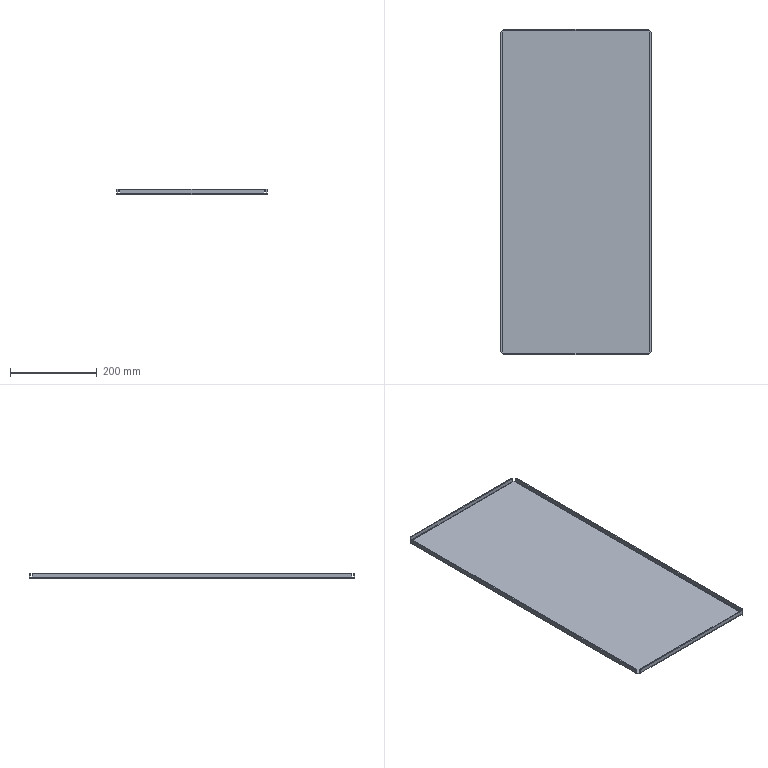Part | SolidWorks | features BaseBody 1 | 1 solid | 50 faces | box 346 x 750 x 12 mm | volume 694682 mm3 | plane 42 | cylinder 8 | commonest cylinder face diameters 1.473 x4 6.473 x4
STEP:
#1=CARTESIAN_POINT('',(-166.,372.5,9.5));
#2=VERTEX_POINT('',#1);
#3=CARTESIAN_POINT('',(166.,372.5,9.5));
#4=VERTEX_POINT('',#3);
#5=CARTESIAN_POINT('',(166.,372.5,9.5));
#6=DIRECTION('',(1.,0.,0.));
#7=VECTOR('',#6,1000.);
#8=LINE('',#5,#7);
#9=EDGE_CURVE('',#2,#4,#8,.T.);
#10=ORIENTED_EDGE('',*,*,#9,.T.);
#11=CARTESIAN_POINT('',(166.,375.,9.5));
#12=VERTEX_POINT('',#11);
#13=CARTESIAN_POINT('',(166.,375.,9.5));
#14=DIRECTION('',(0.,-1.,0.));
#15=VECTOR('',#14,1000.);
#16=LINE('',#13,#15);
#17=EDGE_CURVE('',#12,#4,#16,.T.);
#18=ORIENTED_EDGE('',*,*,#17,.F.);
#19=CARTESIAN_POINT('',(-166.,375.,9.5));
#20=VERTEX_POINT('',#19);
#21=CARTESIAN_POINT('',(0.,375.,9.5));
#22=DIRECTION('',(1.,0.,0.));
#23=VECTOR('',#22,1000.);
#24=LINE('',#21,#23);
#25=EDGE_CURVE('',#20,#12,#24,.T.);
#26=ORIENTED_EDGE('',*,*,#25,.F.);
#27=CARTESIAN_POINT('',(-166.,375.,9.5));
#28=DIRECTION('',(0.,-1.,0.));
#29=VECTOR('',#28,1000.);
#30=LINE('',#27,#29);
#31=EDGE_CURVE('',#20,#2,#30,.T.);
#32=ORIENTED_EDGE('',*,*,#31,.T.);
#33=EDGE_LOOP('',(#10,#18,#26,#32));
#34=FACE_OUTER_BOUND('',#33,.T.);
#35=CARTESIAN_POINT('',(166.,375.,9.5));
#36=DIRECTION('',(0.,0.,-1.));
#37=DIRECTION('',(0.,-1.,0.));
#38=AXIS2_PLACEMENT_3D('',#35,#36,#37);
#39=PLANE('',#38);
#40=ADVANCED_FACE('',(#34),#39,.F.);
#41=CARTESIAN_POINT('',(-166.,372.5,0.7366));
#42=VERTEX_POINT('',#41);
#43=CARTESIAN_POINT('',(-166.,372.5,9.5));
#44=DIRECTION('',(0.,0.,1.));
#45=VECTOR('',#44,1000.);
#46=LINE('',#43,#45);
#47=EDGE_CURVE('',#42,#2,#46,.T.);
#48=ORIENTED_EDGE('',*,*,#47,.F.);
#49=CARTESIAN_POINT('',(166.,372.5,0.7366));
#50=VERTEX_POINT('',#49);
#51=CARTESIAN_POINT('',(166.,372.5,0.7366));
#52=DIRECTION('',(-1.,0.,0.));
#53=VECTOR('',#52,1000.);
#54=LINE('',#51,#53);
#55=EDGE_CURVE('',#50,#42,#54,.T.);
#56=ORIENTED_EDGE('',*,*,#55,.F.);
#57=CARTESIAN_POINT('',(166.,372.5,0.));
#58=DIRECTION('',(0.,0.,-1.));
#59=VECTOR('',#58,1000.);
#60=LINE('',#57,#59);
#61=EDGE_CURVE('',#4,#50,#60,.T.);
#62=ORIENTED_EDGE('',*,*,#61,.F.);
#63=ORIENTED_EDGE('',*,*,#9,.F.);
#64=EDGE_LOOP('',(#48,#56,#62,#63));
#65=FACE_OUTER_BOUND('',#64,.T.);
#66=CARTESIAN_POINT('',(0.,372.5,0.));
#67=DIRECTION('',(0.,-1.,0.));
#68=DIRECTION('',(0.,0.,-1.));
#69=AXIS2_PLACEMENT_3D('',#66,#67,#68);
#70=PLANE('',#69);
#71=ADVANCED_FACE('',(#65),#70,.T.);
#72=CARTESIAN_POINT('',(-166.,375.,0.7366));
#73=VERTEX_POINT('',#72);
#74=CARTESIAN_POINT('',(166.,375.,0.7366));
#75=VERTEX_POINT('',#74);
#76=CARTESIAN_POINT('',(166.,375.,0.7366));
#77=DIRECTION('',(1.,0.,0.));
#78=VECTOR('',#77,1000.);
#79=LINE('',#76,#78);
#80=EDGE_CURVE('',#73,#75,#79,.T.);
#81=ORIENTED_EDGE('',*,*,#80,.F.);
#82=CARTESIAN_POINT('',(-166.,375.,0.));
#83=DIRECTION('',(0.,0.,1.));
#84=VECTOR('',#83,1000.);
#85=LINE('',#82,#84);
#86=EDGE_CURVE('',#73,#20,#85,.T.);
#87=ORIENTED_EDGE('',*,*,#86,.T.);
#88=ORIENTED_EDGE('',*,*,#25,.T.);
#89=CARTESIAN_POINT('',(166.,375.,0.));
#90=DIRECTION('',(0.,0.,-1.));
#91=VECTOR('',#90,1000.);
#92=LINE('',#89,#91);
#93=EDGE_CURVE('',#12,#75,#92,.T.);
#94=ORIENTED_EDGE('',*,*,#93,.T.);
#95=EDGE_LOOP('',(#81,#87,#88,#94));
#96=FACE_OUTER_BOUND('',#95,.T.);
#97=CARTESIAN_POINT('',(0.,375.,0.));
#98=DIRECTION('',(0.,-1.,0.));
#99=DIRECTION('',(0.,0.,-1.));
#100=AXIS2_PLACEMENT_3D('',#97,#98,#99);
#101=PLANE('',#100);
#102=ADVANCED_FACE('',(#96),#101,.F.);
#103=CARTESIAN_POINT('',(-166.,372.5,0.7366));
#104=DIRECTION('',(0.,1.,0.));
#105=VECTOR('',#104,1000.);
#106=LINE('',#103,#105);
#107=EDGE_CURVE('',#42,#73,#106,.T.);
#108=ORIENTED_EDGE('',*,*,#107,.F.);
#109=ORIENTED_EDGE('',*,*,#47,.T.);
#110=ORIENTED_EDGE('',*,*,#31,.F.);
#111=ORIENTED_EDGE('',*,*,#86,.F.);
#112=EDGE_LOOP('',(#108,#109,#110,#111));
#113=FACE_OUTER_BOUND('',#112,.T.);
#114=CARTESIAN_POINT('',(-166.,375.,9.5));
#115=DIRECTION('',(1.,0.,0.));
#116=DIRECTION('',(0.,1.,0.));
#117=AXIS2_PLACEMENT_3D('',#114,#115,#116);
#118=PLANE('',#117);
#119=ADVANCED_FACE('',(#113),#118,.F.);
#120=CARTESIAN_POINT('',(166.,375.,0.7366));
#121=DIRECTION('',(0.,1.,0.));
#122=VECTOR('',#121,1000.);
#123=LINE('',#120,#122);
#124=EDGE_CURVE('',#50,#75,#123,.T.);
#125=ORIENTED_EDGE('',*,*,#124,.T.);
#126=ORIENTED_EDGE('',*,*,#93,.F.);
#127=ORIENTED_EDGE('',*,*,#17,.T.);
#128=ORIENTED_EDGE('',*,*,#61,.T.);
#129=EDGE_LOOP('',(#125,#126,#127,#128));
#130=FACE_OUTER_BOUND('',#129,.T.);
#131=CARTESIAN_POINT('',(166.,375.,0.));
#132=DIRECTION('',(-1.,0.,0.));
#133=DIRECTION('',(0.,1.,0.));
#134=AXIS2_PLACEMENT_3D('',#131,#132,#133);
#135=PLANE('',#134);
#136=ADVANCED_FACE('',(#130),#135,.F.);
#137=CARTESIAN_POINT('',(-166.,371.763,0.));
#138=VERTEX_POINT('',#137);
#139=CARTESIAN_POINT('',(166.,371.763,0.));
#140=VERTEX_POINT('',#139);
#141=CARTESIAN_POINT('',(-166.,371.763,0.));
#142=DIRECTION('',(1.,0.,0.));
#143=VECTOR('',#142,1000.);
#144=LINE('',#141,#143);
#145=EDGE_CURVE('',#138,#140,#144,.T.);
#146=ORIENTED_EDGE('',*,*,#145,.T.);
#147=CARTESIAN_POINT('',(166.,371.763,0.7366));
#148=DIRECTION('',(1.,0.,0.));
#149=DIRECTION('',(0.,0.,1.));
#150=AXIS2_PLACEMENT_3D('',#147,#148,#149);
#151=CIRCLE('',#150,0.7366);
#152=EDGE_CURVE('',#140,#50,#151,.T.);
#153=ORIENTED_EDGE('',*,*,#152,.T.);
#154=ORIENTED_EDGE('',*,*,#55,.T.);
#155=CARTESIAN_POINT('',(-166.,371.763,0.7366));
#156=DIRECTION('',(-1.,0.,0.));
#157=DIRECTION('',(0.,0.,1.));
#158=AXIS2_PLACEMENT_3D('',#155,#156,#157);
#159=CIRCLE('',#158,0.7366);
#160=EDGE_CURVE('',#42,#138,#159,.T.);
#161=ORIENTED_EDGE('',*,*,#160,.T.);
#162=EDGE_LOOP('',(#146,#153,#154,#161));
#163=FACE_OUTER_BOUND('',#162,.T.);
#164=CARTESIAN_POINT('',(-166.,371.763,0.7366));
#165=DIRECTION('',(-1.,0.,0.));
#166=DIRECTION('',(0.,1.,0.));
#167=AXIS2_PLACEMENT_3D('',#164,#165,#166);
#168=CYLINDRICAL_SURFACE('',#167,0.7366);
#169=ADVANCED_FACE('',(#163),#168,.F.);
#170=CARTESIAN_POINT('',(-166.,371.763,-2.5));
#171=VERTEX_POINT('',#170);
#172=CARTESIAN_POINT('',(166.,371.763,-2.5));
#173=VERTEX_POINT('',#172);
#174=CARTESIAN_POINT('',(-166.,371.763,-2.5));
#175=DIRECTION('',(1.,0.,0.));
#176=VECTOR('',#175,1000.);
#177=LINE('',#174,#176);
#178=EDGE_CURVE('',#171,#173,#177,.T.);
#179=ORIENTED_EDGE('',*,*,#178,.F.);
#180=CARTESIAN_POINT('',(-166.,374.915,0.));
#181=VERTEX_POINT('',#180);
#182=CARTESIAN_POINT('',(-166.,371.763,0.7366));
#183=DIRECTION('',(-1.,0.,0.));
#184=DIRECTION('',(0.,0.,1.));
#185=AXIS2_PLACEMENT_3D('',#182,#183,#184);
#186=CIRCLE('',#185,3.237);
#187=EDGE_CURVE('',#181,#171,#186,.T.);
#188=ORIENTED_EDGE('',*,*,#187,.F.);
#189=CARTESIAN_POINT('',(-166.,371.763,0.7366));
#190=DIRECTION('',(-1.,0.,0.));
#191=DIRECTION('',(0.,0.,1.));
#192=AXIS2_PLACEMENT_3D('',#189,#190,#191);
#193=CIRCLE('',#192,3.237);
#194=EDGE_CURVE('',#73,#181,#193,.T.);
#195=ORIENTED_EDGE('',*,*,#194,.F.);
#196=ORIENTED_EDGE('',*,*,#80,.T.);
#197=CARTESIAN_POINT('',(166.,374.915,0.));
#198=VERTEX_POINT('',#197);
#199=CARTESIAN_POINT('',(166.,371.763,0.7366));
#200=DIRECTION('',(1.,0.,0.));
#201=DIRECTION('',(0.,0.,1.));
#202=AXIS2_PLACEMENT_3D('',#199,#200,#201);
#203=CIRCLE('',#202,3.237);
#204=EDGE_CURVE('',#198,#75,#203,.T.);
#205=ORIENTED_EDGE('',*,*,#204,.F.);
#206=CARTESIAN_POINT('',(166.,371.763,0.7366));
#207=DIRECTION('',(1.,0.,0.));
#208=DIRECTION('',(0.,0.,1.));
#209=AXIS2_PLACEMENT_3D('',#206,#207,#208);
#210=CIRCLE('',#209,3.237);
#211=EDGE_CURVE('',#173,#198,#210,.T.);
#212=ORIENTED_EDGE('',*,*,#211,.F.);
#213=EDGE_LOOP('',(#179,#188,#195,#196,#205,#212));
#214=FACE_OUTER_BOUND('',#213,.T.);
#215=CARTESIAN_POINT('',(-166.,371.763,0.7366));
#216=DIRECTION('',(-1.,0.,0.));
#217=DIRECTION('',(0.,1.,0.));
#218=AXIS2_PLACEMENT_3D('',#215,#216,#217);
#219=CYLINDRICAL_SURFACE('',#218,3.237);
#220=ADVANCED_FACE('',(#214),#219,.T.);
#221=ORIENTED_EDGE('',*,*,#194,.T.);
#222=CARTESIAN_POINT('',(-166.,375.,0.));
#223=DIRECTION('',(0.,-1.,0.));
#224=VECTOR('',#223,1000.);
#225=LINE('',#222,#224);
#226=EDGE_CURVE('',#181,#138,#225,.T.);
#227=ORIENTED_EDGE('',*,*,#226,.T.);
#228=ORIENTED_EDGE('',*,*,#160,.F.);
#229=ORIENTED_EDGE('',*,*,#107,.T.);
#230=EDGE_LOOP('',(#221,#227,#228,#229));
#231=FACE_OUTER_BOUND('',#230,.T.);
#232=CARTESIAN_POINT('',(-166.,371.763,0.7366));
#233=DIRECTION('',(1.,0.,0.));
#234=DIRECTION('',(0.,0.,1.));
#235=AXIS2_PLACEMENT_3D('',#232,#233,#234);
#236=PLANE('',#235);
#237=ADVANCED_FACE('',(#231),#236,.F.);
#238=ORIENTED_EDGE('',*,*,#152,.F.);
#239=CARTESIAN_POINT('',(166.,371.763,0.));
#240=DIRECTION('',(0.,1.,0.));
#241=VECTOR('',#240,1000.);
#242=LINE('',#239,#241);
#243=EDGE_CURVE('',#140,#198,#242,.T.);
#244=ORIENTED_EDGE('',*,*,#243,.T.);
#245=ORIENTED_EDGE('',*,*,#204,.T.);
#246=ORIENTED_EDGE('',*,*,#124,.F.);
#247=EDGE_LOOP('',(#238,#244,#245,#246));
#248=FACE_OUTER_BOUND('',#247,.T.);
#249=CARTESIAN_POINT('',(166.,371.763,0.7366));
#250=DIRECTION('',(1.,0.,0.));
#251=DIRECTION('',(0.,0.,1.));
#252=AXIS2_PLACEMENT_3D('',#249,#250,#251);
#253=PLANE('',#252);
#254=ADVANCED_FACE('',(#248),#253,.T.);
#255=CARTESIAN_POINT('',(170.5,368.,9.5));
#256=VERTEX_POINT('',#255);
#257=CARTESIAN_POINT('',(170.5,-368.,9.5));
#258=VERTEX_POINT('',#257);
#259=CARTESIAN_POINT('',(170.5,-368.,9.5));
#260=DIRECTION('',(0.,-1.,0.));
#261=VECTOR('',#260,1000.);
#262=LINE('',#259,#261);
#263=EDGE_CURVE('',#256,#258,#262,.T.);
#264=ORIENTED_EDGE('',*,*,#263,.T.);
#265=CARTESIAN_POINT('',(173.,-368.,9.5));
#266=VERTEX_POINT('',#265);
#267=CARTESIAN_POINT('',(173.,-368.,9.5));
#268=DIRECTION('',(-1.,0.,0.));
#269=VECTOR('',#268,1000.);
#270=LINE('',#267,#269);
#271=EDGE_CURVE('',#266,#258,#270,.T.);
#272=ORIENTED_EDGE('',*,*,#271,.F.);
#273=CARTESIAN_POINT('',(173.,368.,9.5));
#274=VERTEX_POINT('',#273);
#275=CARTESIAN_POINT('',(173.,0.,9.5));
#276=DIRECTION('',(0.,-1.,0.));
#277=VECTOR('',#276,1000.);
#278=LINE('',#275,#277);
#279=EDGE_CURVE('',#274,#266,#278,.T.);
#280=ORIENTED_EDGE('',*,*,#279,.F.);
#281=CARTESIAN_POINT('',(173.,368.,9.5));
#282=DIRECTION('',(-1.,0.,0.));
#283=VECTOR('',#282,1000.);
#284=LINE('',#281,#283);
#285=EDGE_CURVE('',#274,#256,#284,.T.);
#286=ORIENTED_EDGE('',*,*,#285,.T.);
#287=EDGE_LOOP('',(#264,#272,#280,#286));
#288=FACE_OUTER_BOUND('',#287,.T.);
#289=CARTESIAN_POINT('',(173.,-368.,9.5));
#290=DIRECTION('',(0.,0.,-1.));
#291=DIRECTION('',(-1.,0.,0.));
#292=AXIS2_PLACEMENT_3D('',#289,#290,#291);
#293=PLANE('',#292);
#294=ADVANCED_FACE('',(#288),#293,.F.);
#295=CARTESIAN_POINT('',(170.5,368.,0.7366));
#296=VERTEX_POINT('',#295);
#297=CARTESIAN_POINT('',(170.5,368.,9.5));
#298=DIRECTION('',(0.,0.,1.));
#299=VECTOR('',#298,1000.);
#300=LINE('',#297,#299);
#301=EDGE_CURVE('',#296,#256,#300,.T.);
#302=ORIENTED_EDGE('',*,*,#301,.F.);
#303=CARTESIAN_POINT('',(170.5,-368.,0.7366));
#304=VERTEX_POINT('',#303);
#305=CARTESIAN_POINT('',(170.5,-368.,0.7366));
#306=DIRECTION('',(0.,1.,0.));
#307=VECTOR('',#306,1000.);
#308=LINE('',#305,#307);
#309=EDGE_CURVE('',#304,#296,#308,.T.);
#310=ORIENTED_EDGE('',*,*,#309,.F.);
#311=CARTESIAN_POINT('',(170.5,-368.,0.));
#312=DIRECTION('',(0.,0.,-1.));
#313=VECTOR('',#312,1000.);
#314=LINE('',#311,#313);
#315=EDGE_CURVE('',#258,#304,#314,.T.);
#316=ORIENTED_EDGE('',*,*,#315,.F.);
#317=ORIENTED_EDGE('',*,*,#263,.F.);
#318=EDGE_LOOP('',(#302,#310,#316,#317));
#319=FACE_OUTER_BOUND('',#318,.T.);
#320=CARTESIAN_POINT('',(170.5,0.,0.));
#321=DIRECTION('',(-1.,0.,0.));
#322=DIRECTION('',(0.,1.,0.));
#323=AXIS2_PLACEMENT_3D('',#320,#321,#322);
#324=PLANE('',#323);
#325=ADVANCED_FACE('',(#319),#324,.T.);
#326=CARTESIAN_POINT('',(173.,368.,0.7366));
#327=VERTEX_POINT('',#326);
#328=CARTESIAN_POINT('',(173.,-368.,0.7366));
#329=VERTEX_POINT('',#328);
#330=CARTESIAN_POINT('',(173.,-368.,0.7366));
#331=DIRECTION('',(0.,-1.,0.));
#332=VECTOR('',#331,1000.);
#333=LINE('',#330,#332);
#334=EDGE_CURVE('',#327,#329,#333,.T.);
#335=ORIENTED_EDGE('',*,*,#334,.F.);
#336=CARTESIAN_POINT('',(173.,368.,0.));
#337=DIRECTION('',(0.,0.,1.));
#338=VECTOR('',#337,1000.);
#339=LINE('',#336,#338);
#340=EDGE_CURVE('',#327,#274,#339,.T.);
#341=ORIENTED_EDGE('',*,*,#340,.T.);
#342=ORIENTED_EDGE('',*,*,#279,.T.);
#343=CARTESIAN_POINT('',(173.,-368.,0.));
#344=DIRECTION('',(0.,0.,-1.));
#345=VECTOR('',#344,1000.);
#346=LINE('',#343,#345);
#347=EDGE_CURVE('',#266,#329,#346,.T.);
#348=ORIENTED_EDGE('',*,*,#347,.T.);
#349=EDGE_LOOP('',(#335,#341,#342,#348));
#350=FACE_OUTER_BOUND('',#349,.T.);
#351=CARTESIAN_POINT('',(173.,0.,0.));
#352=DIRECTION('',(-1.,0.,0.));
#353=DIRECTION('',(0.,1.,0.));
#354=AXIS2_PLACEMENT_3D('',#351,#352,#353);
#355=PLANE('',#354);
#356=ADVANCED_FACE('',(#350),#355,.F.);
#357=CARTESIAN_POINT('',(170.5,368.,0.7366));
#358=DIRECTION('',(1.,0.,0.));
#359=VECTOR('',#358,1000.);
#360=LINE('',#357,#359);
#361=EDGE_CURVE('',#296,#327,#360,.T.);
#362=ORIENTED_EDGE('',*,*,#361,.F.);
#363=ORIENTED_EDGE('',*,*,#301,.T.);
#364=ORIENTED_EDGE('',*,*,#285,.F.);
#365=ORIENTED_EDGE('',*,*,#340,.F.);
#366=EDGE_LOOP('',(#362,#363,#364,#365));
#367=FACE_OUTER_BOUND('',#366,.T.);
#368=CARTESIAN_POINT('',(173.,368.,9.5));
#369=DIRECTION('',(0.,-1.,0.));
#370=DIRECTION('',(0.,0.,-1.));
#371=AXIS2_PLACEMENT_3D('',#368,#369,#370);
#372=PLANE('',#371);
#373=ADVANCED_FACE('',(#367),#372,.F.);
#374=CARTESIAN_POINT('',(173.,-368.,0.7366));
#375=DIRECTION('',(1.,0.,0.));
#376=VECTOR('',#375,1000.);
#377=LINE('',#374,#376);
#378=EDGE_CURVE('',#304,#329,#377,.T.);
#379=ORIENTED_EDGE('',*,*,#378,.T.);
#380=ORIENTED_EDGE('',*,*,#347,.F.);
#381=ORIENTED_EDGE('',*,*,#271,.T.);
#382=ORIENTED_EDGE('',*,*,#315,.T.);
#383=EDGE_LOOP('',(#379,#380,#381,#382));
#384=FACE_OUTER_BOUND('',#383,.T.);
#385=CARTESIAN_POINT('',(173.,-368.,0.));
#386=DIRECTION('',(0.,1.,0.));
#387=DIRECTION('',(0.,0.,-1.));
#388=AXIS2_PLACEMENT_3D('',#385,#386,#387);
#389=PLANE('',#388);
#390=ADVANCED_FACE('',(#384),#389,.F.);
#391=CARTESIAN_POINT('',(169.763,368.,0.));
#392=VERTEX_POINT('',#391);
#393=CARTESIAN_POINT('',(169.763,-368.,0.));
#394=VERTEX_POINT('',#393);
#395=CARTESIAN_POINT('',(169.763,368.,0.));
#396=DIRECTION('',(0.,-1.,0.));
#397=VECTOR('',#396,1000.);
#398=LINE('',#395,#397);
#399=EDGE_CURVE('',#392,#394,#398,.T.);
#400=ORIENTED_EDGE('',*,*,#399,.T.);
#401=CARTESIAN_POINT('',(169.763,-368.,0.7366));
#402=DIRECTION('',(0.,-1.,0.));
#403=DIRECTION('',(0.,0.,1.));
#404=AXIS2_PLACEMENT_3D('',#401,#402,#403);
#405=CIRCLE('',#404,0.7366);
#406=EDGE_CURVE('',#394,#304,#405,.T.);
#407=ORIENTED_EDGE('',*,*,#406,.T.);
#408=ORIENTED_EDGE('',*,*,#309,.T.);
#409=CARTESIAN_POINT('',(169.763,368.,0.7366));
#410=DIRECTION('',(0.,1.,0.));
#411=DIRECTION('',(0.,0.,1.));
#412=AXIS2_PLACEMENT_3D('',#409,#410,#411);
#413=CIRCLE('',#412,0.7366);
#414=EDGE_CURVE('',#296,#392,#413,.T.);
#415=ORIENTED_EDGE('',*,*,#414,.T.);
#416=EDGE_LOOP('',(#400,#407,#408,#415));
#417=FACE_OUTER_BOUND('',#416,.T.);
#418=CARTESIAN_POINT('',(169.763,368.,0.7366));
#419=DIRECTION('',(0.,1.,0.));
#420=DIRECTION('',(1.,0.,0.));
#421=AXIS2_PLACEMENT_3D('',#418,#419,#420);
#422=CYLINDRICAL_SURFACE('',#421,0.7366);
#423=ADVANCED_FACE('',(#417),#422,.F.);
#424=CARTESIAN_POINT('',(169.763,368.,-2.5));
#425=VERTEX_POINT('',#424);
#426=CARTESIAN_POINT('',(169.763,-368.,-2.5));
#427=VERTEX_POINT('',#426);
#428=CARTESIAN_POINT('',(169.763,368.,-2.5));
#429=DIRECTION('',(0.,-1.,0.));
#430=VECTOR('',#429,1000.);
#431=LINE('',#428,#430);
#432=EDGE_CURVE('',#425,#427,#431,.T.);
#433=ORIENTED_EDGE('',*,*,#432,.F.);
#434=CARTESIAN_POINT('',(172.915,368.,0.));
#435=VERTEX_POINT('',#434);
#436=CARTESIAN_POINT('',(169.763,368.,0.7366));
#437=DIRECTION('',(0.,1.,0.));
#438=DIRECTION('',(0.,0.,1.));
#439=AXIS2_PLACEMENT_3D('',#436,#437,#438);
#440=CIRCLE('',#439,3.237);
#441=EDGE_CURVE('',#435,#425,#440,.T.);
#442=ORIENTED_EDGE('',*,*,#441,.F.);
#443=CARTESIAN_POINT('',(169.763,368.,0.7366));
#444=DIRECTION('',(0.,1.,0.));
#445=DIRECTION('',(0.,0.,1.));
#446=AXIS2_PLACEMENT_3D('',#443,#444,#445);
#447=CIRCLE('',#446,3.237);
#448=EDGE_CURVE('',#327,#435,#447,.T.);
#449=ORIENTED_EDGE('',*,*,#448,.F.);
#450=ORIENTED_EDGE('',*,*,#334,.T.);
#451=CARTESIAN_POINT('',(172.915,-368.,0.));
#452=VERTEX_POINT('',#451);
#453=CARTESIAN_POINT('',(169.763,-368.,0.7366));
#454=DIRECTION('',(0.,-1.,0.));
#455=DIRECTION('',(0.,0.,1.));
#456=AXIS2_PLACEMENT_3D('',#453,#454,#455);
#457=CIRCLE('',#456,3.237);
#458=EDGE_CURVE('',#452,#329,#457,.T.);
#459=ORIENTED_EDGE('',*,*,#458,.F.);
#460=CARTESIAN_POINT('',(169.763,-368.,0.7366));
#461=DIRECTION('',(0.,-1.,0.));
#462=DIRECTION('',(0.,0.,1.));
#463=AXIS2_PLACEMENT_3D('',#460,#461,#462);
#464=CIRCLE('',#463,3.237);
#465=EDGE_CURVE('',#427,#452,#464,.T.);
#466=ORIENTED_EDGE('',*,*,#465,.F.);
#467=EDGE_LOOP('',(#433,#442,#449,#450,#459,#466));
#468=FACE_OUTER_BOUND('',#467,.T.);
#469=CARTESIAN_POINT('',(169.763,368.,0.7366));
#470=DIRECTION('',(0.,1.,0.));
#471=DIRECTION('',(1.,0.,0.));
#472=AXIS2_PLACEMENT_3D('',#469,#470,#471);
#473=CYLINDRICAL_SURFACE('',#472,3.237);
#474=ADVANCED_FACE('',(#468),#473,.T.);
#475=ORIENTED_EDGE('',*,*,#448,.T.);
#476=CARTESIAN_POINT('',(173.,368.,0.));
#477=DIRECTION('',(-1.,0.,0.));
#478=VECTOR('',#477,1000.);
#479=LINE('',#476,#478);
#480=EDGE_CURVE('',#435,#392,#479,.T.);
#481=ORIENTED_EDGE('',*,*,#480,.T.);
#482=ORIENTED_EDGE('',*,*,#414,.F.);
#483=ORIENTED_EDGE('',*,*,#361,.T.);
#484=EDGE_LOOP('',(#475,#481,#482,#483));
#485=FACE_OUTER_BOUND('',#484,.T.);
#486=CARTESIAN_POINT('',(169.763,368.,0.7366));
#487=DIRECTION('',(0.,-1.,0.));
#488=DIRECTION('',(-1.,0.,0.));
#489=AXIS2_PLACEMENT_3D('',#486,#487,#488);
#490=PLANE('',#489);
#491=ADVANCED_FACE('',(#485),#490,.F.);
#492=ORIENTED_EDGE('',*,*,#406,.F.);
#493=CARTESIAN_POINT('',(169.763,-368.,0.));
#494=DIRECTION('',(1.,0.,0.));
#495=VECTOR('',#494,1000.);
#496=LINE('',#493,#495);
#497=EDGE_CURVE('',#394,#452,#496,.T.);
#498=ORIENTED_EDGE('',*,*,#497,.T.);
#499=ORIENTED_EDGE('',*,*,#458,.T.);
#500=ORIENTED_EDGE('',*,*,#378,.F.);
#501=EDGE_LOOP('',(#492,#498,#499,#500));
#502=FACE_OUTER_BOUND('',#501,.T.);
#503=CARTESIAN_POINT('',(169.763,-368.,0.7366));
#504=DIRECTION('',(0.,-1.,0.));
#505=DIRECTION('',(-1.,0.,0.));
#506=AXIS2_PLACEMENT_3D('',#503,#504,#505);
#507=PLANE('',#506);
#508=ADVANCED_FACE('',(#502),#507,.T.);
#509=CARTESIAN_POINT('',(166.,-372.5,9.5));
#510=VERTEX_POINT('',#509);
#511=CARTESIAN_POINT('',(-166.,-372.5,9.5));
#512=VERTEX_POINT('',#511);
#513=CARTESIAN_POINT('',(-166.,-372.5,9.5));
#514=DIRECTION('',(-1.,0.,0.));
#515=VECTOR('',#514,1000.);
#516=LINE('',#513,#515);
#517=EDGE_CURVE('',#510,#512,#516,.T.);
#518=ORIENTED_EDGE('',*,*,#517,.T.);
#519=CARTESIAN_POINT('',(-166.,-375.,9.5));
#520=VERTEX_POINT('',#519);
#521=CARTESIAN_POINT('',(-166.,-375.,9.5));
#522=DIRECTION('',(0.,1.,0.));
#523=VECTOR('',#522,1000.);
#524=LINE('',#521,#523);
#525=EDGE_CURVE('',#520,#512,#524,.T.);
#526=ORIENTED_EDGE('',*,*,#525,.F.);
#527=CARTESIAN_POINT('',(166.,-375.,9.5));
#528=VERTEX_POINT('',#527);
#529=CARTESIAN_POINT('',(0.,-375.,9.5));
#530=DIRECTION('',(-1.,0.,0.));
#531=VECTOR('',#530,1000.);
#532=LINE('',#529,#531);
#533=EDGE_CURVE('',#528,#520,#532,.T.);
#534=ORIENTED_EDGE('',*,*,#533,.F.);
#535=CARTESIAN_POINT('',(166.,-375.,9.5));
#536=DIRECTION('',(0.,1.,0.));
#537=VECTOR('',#536,1000.);
#538=LINE('',#535,#537);
#539=EDGE_CURVE('',#528,#510,#538,.T.);
#540=ORIENTED_EDGE('',*,*,#539,.T.);
#541=EDGE_LOOP('',(#518,#526,#534,#540));
#542=FACE_OUTER_BOUND('',#541,.T.);
#543=CARTESIAN_POINT('',(-166.,-375.,9.5));
#544=DIRECTION('',(0.,0.,-1.));
#545=DIRECTION('',(-1.,0.,0.));
#546=AXIS2_PLACEMENT_3D('',#543,#544,#545);
#547=PLANE('',#546);
#548=ADVANCED_FACE('',(#542),#547,.F.);
#549=CARTESIAN_POINT('',(166.,-372.5,0.7366));
#550=VERTEX_POINT('',#549);
#551=CARTESIAN_POINT('',(166.,-372.5,9.5));
#552=DIRECTION('',(0.,0.,1.));
#553=VECTOR('',#552,1000.);
#554=LINE('',#551,#553);
#555=EDGE_CURVE('',#550,#510,#554,.T.);
#556=ORIENTED_EDGE('',*,*,#555,.F.);
#557=CARTESIAN_POINT('',(-166.,-372.5,0.7366));
#558=VERTEX_POINT('',#557);
#559=CARTESIAN_POINT('',(-166.,-372.5,0.7366));
#560=DIRECTION('',(1.,0.,0.));
#561=VECTOR('',#560,1000.);
#562=LINE('',#559,#561);
#563=EDGE_CURVE('',#558,#550,#562,.T.);
#564=ORIENTED_EDGE('',*,*,#563,.F.);
#565=CARTESIAN_POINT('',(-166.,-372.5,0.));
#566=DIRECTION('',(0.,0.,-1.));
#567=VECTOR('',#566,1000.);
#568=LINE('',#565,#567);
#569=EDGE_CURVE('',#512,#558,#568,.T.);
#570=ORIENTED_EDGE('',*,*,#569,.F.);
#571=ORIENTED_EDGE('',*,*,#517,.F.);
#572=EDGE_LOOP('',(#556,#564,#570,#571));
#573=FACE_OUTER_BOUND('',#572,.T.);
#574=CARTESIAN_POINT('',(0.,-372.5,0.));
#575=DIRECTION('',(0.,1.,0.));
#576=DIRECTION('',(0.,0.,-1.));
#577=AXIS2_PLACEMENT_3D('',#574,#575,#576);
#578=PLANE('',#577);
#579=ADVANCED_FACE('',(#573),#578,.T.);
#580=CARTESIAN_POINT('',(166.,-375.,0.7366));
#581=VERTEX_POINT('',#580);
#582=CARTESIAN_POINT('',(-166.,-375.,0.7366));
#583=VERTEX_POINT('',#582);
#584=CARTESIAN_POINT('',(-166.,-375.,0.7366));
#585=DIRECTION('',(-1.,0.,0.));
#586=VECTOR('',#585,1000.);
#587=LINE('',#584,#586);
#588=EDGE_CURVE('',#581,#583,#587,.T.);
#589=ORIENTED_EDGE('',*,*,#588,.F.);
#590=CARTESIAN_POINT('',(166.,-375.,0.));
#591=DIRECTION('',(0.,0.,1.));
#592=VECTOR('',#591,1000.);
#593=LINE('',#590,#592);
#594=EDGE_CURVE('',#581,#528,#593,.T.);
#595=ORIENTED_EDGE('',*,*,#594,.T.);
#596=ORIENTED_EDGE('',*,*,#533,.T.);
#597=CARTESIAN_POINT('',(-166.,-375.,0.));
#598=DIRECTION('',(0.,0.,-1.));
#599=VECTOR('',#598,1000.);
#600=LINE('',#597,#599);
#601=EDGE_CURVE('',#520,#583,#600,.T.);
#602=ORIENTED_EDGE('',*,*,#601,.T.);
#603=EDGE_LOOP('',(#589,#595,#596,#602));
#604=FACE_OUTER_BOUND('',#603,.T.);
#605=CARTESIAN_POINT('',(0.,-375.,0.));
#606=DIRECTION('',(0.,1.,0.));
#607=DIRECTION('',(0.,0.,-1.));
#608=AXIS2_PLACEMENT_3D('',#605,#606,#607);
#609=PLANE('',#608);
#610=ADVANCED_FACE('',(#604),#609,.F.);
#611=CARTESIAN_POINT('',(166.,-372.5,0.7366));
#612=DIRECTION('',(0.,-1.,0.));
#613=VECTOR('',#612,1000.);
#614=LINE('',#611,#613);
#615=EDGE_CURVE('',#550,#581,#614,.T.);
#616=ORIENTED_EDGE('',*,*,#615,.F.);
#617=ORIENTED_EDGE('',*,*,#555,.T.);
#618=ORIENTED_EDGE('',*,*,#539,.F.);
#619=ORIENTED_EDGE('',*,*,#594,.F.);
#620=EDGE_LOOP('',(#616,#617,#618,#619));
#621=FACE_OUTER_BOUND('',#620,.T.);
#622=CARTESIAN_POINT('',(166.,-375.,9.5));
#623=DIRECTION('',(-1.,0.,0.));
#624=DIRECTION('',(0.,1.,0.));
#625=AXIS2_PLACEMENT_3D('',#622,#623,#624);
#626=PLANE('',#625);
#627=ADVANCED_FACE('',(#621),#626,.F.);
#628=CARTESIAN_POINT('',(-166.,-375.,0.7366));
#629=DIRECTION('',(0.,-1.,0.));
#630=VECTOR('',#629,1000.);
#631=LINE('',#628,#630);
#632=EDGE_CURVE('',#558,#583,#631,.T.);
#633=ORIENTED_EDGE('',*,*,#632,.T.);
#634=ORIENTED_EDGE('',*,*,#601,.F.);
#635=ORIENTED_EDGE('',*,*,#525,.T.);
#636=ORIENTED_EDGE('',*,*,#569,.T.);
#637=EDGE_LOOP('',(#633,#634,#635,#636));
#638=FACE_OUTER_BOUND('',#637,.T.);
#639=CARTESIAN_POINT('',(-166.,-375.,0.));
#640=DIRECTION('',(1.,0.,0.));
#641=DIRECTION('',(0.,1.,0.));
#642=AXIS2_PLACEMENT_3D('',#639,#640,#641);
#643=PLANE('',#642);
#644=ADVANCED_FACE('',(#638),#643,.F.);
#645=CARTESIAN_POINT('',(166.,-371.763,0.));
#646=VERTEX_POINT('',#645);
#647=CARTESIAN_POINT('',(-166.,-371.763,0.));
#648=VERTEX_POINT('',#647);
#649=CARTESIAN_POINT('',(166.,-371.763,0.));
#650=DIRECTION('',(-1.,0.,0.));
#651=VECTOR('',#650,1000.);
#652=LINE('',#649,#651);
#653=EDGE_CURVE('',#646,#648,#652,.T.);
#654=ORIENTED_EDGE('',*,*,#653,.T.);
#655=CARTESIAN_POINT('',(-166.,-371.763,0.7366));
#656=DIRECTION('',(-1.,0.,0.));
#657=DIRECTION('',(0.,0.,-1.));
#658=AXIS2_PLACEMENT_3D('',#655,#656,#657);
#659=CIRCLE('',#658,0.7366);
#660=EDGE_CURVE('',#648,#558,#659,.T.);
#661=ORIENTED_EDGE('',*,*,#660,.T.);
#662=ORIENTED_EDGE('',*,*,#563,.T.);
#663=CARTESIAN_POINT('',(166.,-371.763,0.7366));
#664=DIRECTION('',(1.,0.,0.));
#665=DIRECTION('',(0.,0.,-1.));
#666=AXIS2_PLACEMENT_3D('',#663,#664,#665);
#667=CIRCLE('',#666,0.7366);
#668=EDGE_CURVE('',#550,#646,#667,.T.);
#669=ORIENTED_EDGE('',*,*,#668,.T.);
#670=EDGE_LOOP('',(#654,#661,#662,#669));
#671=FACE_OUTER_BOUND('',#670,.T.);
#672=CARTESIAN_POINT('',(166.,-371.763,0.7366));
#673=DIRECTION('',(1.,0.,0.));
#674=DIRECTION('',(0.,-1.,0.));
#675=AXIS2_PLACEMENT_3D('',#672,#673,#674);
#676=CYLINDRICAL_SURFACE('',#675,0.7366);
#677=ADVANCED_FACE('',(#671),#676,.F.);
#678=CARTESIAN_POINT('',(166.,-371.763,-2.5));
#679=VERTEX_POINT('',#678);
#680=CARTESIAN_POINT('',(-166.,-371.763,-2.5));
#681=VERTEX_POINT('',#680);
#682=CARTESIAN_POINT('',(166.,-371.763,-2.5));
#683=DIRECTION('',(-1.,0.,0.));
#684=VECTOR('',#683,1000.);
#685=LINE('',#682,#684);
#686=EDGE_CURVE('',#679,#681,#685,.T.);
#687=ORIENTED_EDGE('',*,*,#686,.F.);
#688=CARTESIAN_POINT('',(166.,-374.915,0.));
#689=VERTEX_POINT('',#688);
#690=CARTESIAN_POINT('',(166.,-371.763,0.7366));
#691=DIRECTION('',(1.,0.,0.));
#692=DIRECTION('',(0.,0.,-1.));
#693=AXIS2_PLACEMENT_3D('',#690,#691,#692);
#694=CIRCLE('',#693,3.237);
#695=EDGE_CURVE('',#689,#679,#694,.T.);
#696=ORIENTED_EDGE('',*,*,#695,.F.);
#697=CARTESIAN_POINT('',(166.,-371.763,0.7366));
#698=DIRECTION('',(1.,0.,0.));
#699=DIRECTION('',(0.,0.,-1.));
#700=AXIS2_PLACEMENT_3D('',#697,#698,#699);
#701=CIRCLE('',#700,3.237);
#702=EDGE_CURVE('',#581,#689,#701,.T.);
#703=ORIENTED_EDGE('',*,*,#702,.F.);
#704=ORIENTED_EDGE('',*,*,#588,.T.);
#705=CARTESIAN_POINT('',(-166.,-374.915,0.));
#706=VERTEX_POINT('',#705);
#707=CARTESIAN_POINT('',(-166.,-371.763,0.7366));
#708=DIRECTION('',(-1.,0.,0.));
#709=DIRECTION('',(0.,0.,-1.));
#710=AXIS2_PLACEMENT_3D('',#707,#708,#709);
#711=CIRCLE('',#710,3.237);
#712=EDGE_CURVE('',#706,#583,#711,.T.);
#713=ORIENTED_EDGE('',*,*,#712,.F.);
#714=CARTESIAN_POINT('',(-166.,-371.763,0.7366));
#715=DIRECTION('',(-1.,0.,0.));
#716=DIRECTION('',(0.,0.,-1.));
#717=AXIS2_PLACEMENT_3D('',#714,#715,#716);
#718=CIRCLE('',#717,3.237);
#719=EDGE_CURVE('',#681,#706,#718,.T.);
#720=ORIENTED_EDGE('',*,*,#719,.F.);
#721=EDGE_LOOP('',(#687,#696,#703,#704,#713,#720));
#722=FACE_OUTER_BOUND('',#721,.T.);
#723=CARTESIAN_POINT('',(166.,-371.763,0.7366));
#724=DIRECTION('',(1.,0.,0.));
#725=DIRECTION('',(0.,-1.,0.));
#726=AXIS2_PLACEMENT_3D('',#723,#724,#725);
#727=CYLINDRICAL_SURFACE('',#726,3.237);
#728=ADVANCED_FACE('',(#722),#727,.T.);
#729=ORIENTED_EDGE('',*,*,#702,.T.);
#730=CARTESIAN_POINT('',(166.,-375.,0.));
#731=DIRECTION('',(0.,1.,0.));
#732=VECTOR('',#731,1000.);
#733=LINE('',#730,#732);
#734=EDGE_CURVE('',#689,#646,#733,.T.);
#735=ORIENTED_EDGE('',*,*,#734,.T.);
#736=ORIENTED_EDGE('',*,*,#668,.F.);
#737=ORIENTED_EDGE('',*,*,#615,.T.);
#738=EDGE_LOOP('',(#729,#735,#736,#737));
#739=FACE_OUTER_BOUND('',#738,.T.);
#740=CARTESIAN_POINT('',(166.,-371.763,0.7366));
#741=DIRECTION('',(-1.,0.,0.));
#742=DIRECTION('',(0.,1.,0.));
#743=AXIS2_PLACEMENT_3D('',#740,#741,#742);
#744=PLANE('',#743);
#745=ADVANCED_FACE('',(#739),#744,.F.);
#746=ORIENTED_EDGE('',*,*,#660,.F.);
#747=CARTESIAN_POINT('',(-166.,-371.763,0.));
#748=DIRECTION('',(0.,-1.,0.));
#749=VECTOR('',#748,1000.);
#750=LINE('',#747,#749);
#751=EDGE_CURVE('',#648,#706,#750,.T.);
#752=ORIENTED_EDGE('',*,*,#751,.T.);
#753=ORIENTED_EDGE('',*,*,#712,.T.);
#754=ORIENTED_EDGE('',*,*,#632,.F.);
#755=EDGE_LOOP('',(#746,#752,#753,#754));
#756=FACE_OUTER_BOUND('',#755,.T.);
#757=CARTESIAN_POINT('',(-166.,-371.763,0.7366));
#758=DIRECTION('',(-1.,0.,0.));
#759=DIRECTION('',(0.,1.,0.));
#760=AXIS2_PLACEMENT_3D('',#757,#758,#759);
#761=PLANE('',#760);
#762=ADVANCED_FACE('',(#756),#761,.T.);
#763=CARTESIAN_POINT('',(-170.5,-368.,9.5));
#764=VERTEX_POINT('',#763);
#765=CARTESIAN_POINT('',(-170.5,368.,9.5));
#766=VERTEX_POINT('',#765);
#767=CARTESIAN_POINT('',(-170.5,368.,9.5));
#768=DIRECTION('',(0.,1.,0.));
#769=VECTOR('',#768,1000.);
#770=LINE('',#767,#769);
#771=EDGE_CURVE('',#764,#766,#770,.T.);
#772=ORIENTED_EDGE('',*,*,#771,.T.);
#773=CARTESIAN_POINT('',(-173.,368.,9.5));
#774=VERTEX_POINT('',#773);
#775=CARTESIAN_POINT('',(-173.,368.,9.5));
#776=DIRECTION('',(1.,0.,0.));
#777=VECTOR('',#776,1000.);
#778=LINE('',#775,#777);
#779=EDGE_CURVE('',#774,#766,#778,.T.);
#780=ORIENTED_EDGE('',*,*,#779,.F.);
#781=CARTESIAN_POINT('',(-173.,-368.,9.5));
#782=VERTEX_POINT('',#781);
#783=CARTESIAN_POINT('',(-173.,0.,9.5));
#784=DIRECTION('',(0.,1.,0.));
#785=VECTOR('',#784,1000.);
#786=LINE('',#783,#785);
#787=EDGE_CURVE('',#782,#774,#786,.T.);
#788=ORIENTED_EDGE('',*,*,#787,.F.);
#789=CARTESIAN_POINT('',(-173.,-368.,9.5));
#790=DIRECTION('',(1.,0.,0.));
#791=VECTOR('',#790,1000.);
#792=LINE('',#789,#791);
#793=EDGE_CURVE('',#782,#764,#792,.T.);
#794=ORIENTED_EDGE('',*,*,#793,.T.);
#795=EDGE_LOOP('',(#772,#780,#788,#794));
#796=FACE_OUTER_BOUND('',#795,.T.);
#797=CARTESIAN_POINT('',(-173.,368.,9.5));
#798=DIRECTION('',(0.,0.,-1.));
#799=DIRECTION('',(0.,-1.,0.));
#800=AXIS2_PLACEMENT_3D('',#797,#798,#799);
#801=PLANE('',#800);
#802=ADVANCED_FACE('',(#796),#801,.F.);
#803=CARTESIAN_POINT('',(-170.5,-368.,0.7366));
#804=VERTEX_POINT('',#803);
#805=CARTESIAN_POINT('',(-170.5,-368.,9.5));
#806=DIRECTION('',(0.,0.,1.));
#807=VECTOR('',#806,1000.);
#808=LINE('',#805,#807);
#809=EDGE_CURVE('',#804,#764,#808,.T.);
#810=ORIENTED_EDGE('',*,*,#809,.F.);
#811=CARTESIAN_POINT('',(-170.5,368.,0.7366));
#812=VERTEX_POINT('',#811);
#813=CARTESIAN_POINT('',(-170.5,368.,0.7366));
#814=DIRECTION('',(0.,-1.,0.));
#815=VECTOR('',#814,1000.);
#816=LINE('',#813,#815);
#817=EDGE_CURVE('',#812,#804,#816,.T.);
#818=ORIENTED_EDGE('',*,*,#817,.F.);
#819=CARTESIAN_POINT('',(-170.5,368.,0.));
#820=DIRECTION('',(0.,0.,-1.));
#821=VECTOR('',#820,1000.);
#822=LINE('',#819,#821);
#823=EDGE_CURVE('',#766,#812,#822,.T.);
#824=ORIENTED_EDGE('',*,*,#823,.F.);
#825=ORIENTED_EDGE('',*,*,#771,.F.);
#826=EDGE_LOOP('',(#810,#818,#824,#825));
#827=FACE_OUTER_BOUND('',#826,.T.);
#828=CARTESIAN_POINT('',(-170.5,0.,0.));
#829=DIRECTION('',(1.,0.,0.));
#830=DIRECTION('',(0.,0.,1.));
#831=AXIS2_PLACEMENT_3D('',#828,#829,#830);
#832=PLANE('',#831);
#833=ADVANCED_FACE('',(#827),#832,.T.);
#834=CARTESIAN_POINT('',(-173.,-368.,0.7366));
#835=VERTEX_POINT('',#834);
#836=CARTESIAN_POINT('',(-173.,368.,0.7366));
#837=VERTEX_POINT('',#836);
#838=CARTESIAN_POINT('',(-173.,368.,0.7366));
#839=DIRECTION('',(0.,1.,0.));
#840=VECTOR('',#839,1000.);
#841=LINE('',#838,#840);
#842=EDGE_CURVE('',#835,#837,#841,.T.);
#843=ORIENTED_EDGE('',*,*,#842,.F.);
#844=CARTESIAN_POINT('',(-173.,-368.,0.));
#845=DIRECTION('',(0.,0.,1.));
#846=VECTOR('',#845,1000.);
#847=LINE('',#844,#846);
#848=EDGE_CURVE('',#835,#782,#847,.T.);
#849=ORIENTED_EDGE('',*,*,#848,.T.);
#850=ORIENTED_EDGE('',*,*,#787,.T.);
#851=CARTESIAN_POINT('',(-173.,368.,0.));
#852=DIRECTION('',(0.,0.,-1.));
#853=VECTOR('',#852,1000.);
#854=LINE('',#851,#853);
#855=EDGE_CURVE('',#774,#837,#854,.T.);
#856=ORIENTED_EDGE('',*,*,#855,.T.);
#857=EDGE_LOOP('',(#843,#849,#850,#856));
#858=FACE_OUTER_BOUND('',#857,.T.);
#859=CARTESIAN_POINT('',(-173.,0.,0.));
#860=DIRECTION('',(1.,0.,0.));
#861=DIRECTION('',(0.,0.,1.));
#862=AXIS2_PLACEMENT_3D('',#859,#860,#861);
#863=PLANE('',#862);
#864=ADVANCED_FACE('',(#858),#863,.F.);
#865=CARTESIAN_POINT('',(-173.,368.,0.7366));
#866=DIRECTION('',(-1.,0.,0.));
#867=VECTOR('',#866,1000.);
#868=LINE('',#865,#867);
#869=EDGE_CURVE('',#812,#837,#868,.T.);
#870=ORIENTED_EDGE('',*,*,#869,.T.);
#871=ORIENTED_EDGE('',*,*,#855,.F.);
#872=ORIENTED_EDGE('',*,*,#779,.T.);
#873=ORIENTED_EDGE('',*,*,#823,.T.);
#874=EDGE_LOOP('',(#870,#871,#872,#873));
#875=FACE_OUTER_BOUND('',#874,.T.);
#876=CARTESIAN_POINT('',(-173.,368.,0.));
#877=DIRECTION('',(0.,-1.,0.));
#878=DIRECTION('',(-1.,0.,0.));
#879=AXIS2_PLACEMENT_3D('',#876,#877,#878);
#880=PLANE('',#879);
#881=ADVANCED_FACE('',(#875),#880,.F.);
#882=CARTESIAN_POINT('',(-170.5,-368.,0.7366));
#883=DIRECTION('',(-1.,0.,0.));
#884=VECTOR('',#883,1000.);
#885=LINE('',#882,#884);
#886=EDGE_CURVE('',#804,#835,#885,.T.);
#887=ORIENTED_EDGE('',*,*,#886,.F.);
#888=ORIENTED_EDGE('',*,*,#809,.T.);
#889=ORIENTED_EDGE('',*,*,#793,.F.);
#890=ORIENTED_EDGE('',*,*,#848,.F.);
#891=EDGE_LOOP('',(#887,#888,#889,#890));
#892=FACE_OUTER_BOUND('',#891,.T.);
#893=CARTESIAN_POINT('',(-173.,-368.,9.5));
#894=DIRECTION('',(0.,1.,0.));
#895=DIRECTION('',(0.,0.,-1.));
#896=AXIS2_PLACEMENT_3D('',#893,#894,#895);
#897=PLANE('',#896);
#898=ADVANCED_FACE('',(#892),#897,.F.);
#899=CARTESIAN_POINT('',(-169.763,-368.,0.));
#900=VERTEX_POINT('',#899);
#901=CARTESIAN_POINT('',(-169.763,368.,0.));
#902=VERTEX_POINT('',#901);
#903=CARTESIAN_POINT('',(-169.763,-368.,0.));
#904=DIRECTION('',(0.,1.,0.));
#905=VECTOR('',#904,1000.);
#906=LINE('',#903,#905);
#907=EDGE_CURVE('',#900,#902,#906,.T.);
#908=ORIENTED_EDGE('',*,*,#907,.T.);
#909=CARTESIAN_POINT('',(-169.763,368.,0.7366));
#910=DIRECTION('',(0.,1.,0.));
#911=DIRECTION('',(0.,0.,-1.));
#912=AXIS2_PLACEMENT_3D('',#909,#910,#911);
#913=CIRCLE('',#912,0.7366);
#914=EDGE_CURVE('',#902,#812,#913,.T.);
#915=ORIENTED_EDGE('',*,*,#914,.T.);
#916=ORIENTED_EDGE('',*,*,#817,.T.);
#917=CARTESIAN_POINT('',(-169.763,-368.,0.7366));
#918=DIRECTION('',(0.,-1.,0.));
#919=DIRECTION('',(0.,0.,-1.));
#920=AXIS2_PLACEMENT_3D('',#917,#918,#919);
#921=CIRCLE('',#920,0.7366);
#922=EDGE_CURVE('',#804,#900,#921,.T.);
#923=ORIENTED_EDGE('',*,*,#922,.T.);
#924=EDGE_LOOP('',(#908,#915,#916,#923));
#925=FACE_OUTER_BOUND('',#924,.T.);
#926=CARTESIAN_POINT('',(-169.763,-368.,0.7366));
#927=DIRECTION('',(0.,-1.,0.));
#928=DIRECTION('',(-1.,0.,0.));
#929=AXIS2_PLACEMENT_3D('',#926,#927,#928);
#930=CYLINDRICAL_SURFACE('',#929,0.7366);
#931=ADVANCED_FACE('',(#925),#930,.F.);
#932=CARTESIAN_POINT('',(-169.763,-368.,-2.5));
#933=VERTEX_POINT('',#932);
#934=CARTESIAN_POINT('',(-169.763,368.,-2.5));
#935=VERTEX_POINT('',#934);
#936=CARTESIAN_POINT('',(-169.763,-368.,-2.5));
#937=DIRECTION('',(0.,1.,0.));
#938=VECTOR('',#937,1000.);
#939=LINE('',#936,#938);
#940=EDGE_CURVE('',#933,#935,#939,.T.);
#941=ORIENTED_EDGE('',*,*,#940,.F.);
#942=CARTESIAN_POINT('',(-172.915,-368.,0.));
#943=VERTEX_POINT('',#942);
#944=CARTESIAN_POINT('',(-169.763,-368.,0.7366));
#945=DIRECTION('',(0.,-1.,0.));
#946=DIRECTION('',(0.,0.,-1.));
#947=AXIS2_PLACEMENT_3D('',#944,#945,#946);
#948=CIRCLE('',#947,3.237);
#949=EDGE_CURVE('',#943,#933,#948,.T.);
#950=ORIENTED_EDGE('',*,*,#949,.F.);
#951=CARTESIAN_POINT('',(-169.763,-368.,0.7366));
#952=DIRECTION('',(0.,-1.,0.));
#953=DIRECTION('',(0.,0.,-1.));
#954=AXIS2_PLACEMENT_3D('',#951,#952,#953);
#955=CIRCLE('',#954,3.237);
#956=EDGE_CURVE('',#835,#943,#955,.T.);
#957=ORIENTED_EDGE('',*,*,#956,.F.);
#958=ORIENTED_EDGE('',*,*,#842,.T.);
#959=CARTESIAN_POINT('',(-172.915,368.,0.));
#960=VERTEX_POINT('',#959);
#961=CARTESIAN_POINT('',(-169.763,368.,0.7366));
#962=DIRECTION('',(0.,1.,0.));
#963=DIRECTION('',(0.,0.,-1.));
#964=AXIS2_PLACEMENT_3D('',#961,#962,#963);
#965=CIRCLE('',#964,3.237);
#966=EDGE_CURVE('',#960,#837,#965,.T.);
#967=ORIENTED_EDGE('',*,*,#966,.F.);
#968=CARTESIAN_POINT('',(-169.763,368.,0.7366));
#969=DIRECTION('',(0.,1.,0.));
#970=DIRECTION('',(0.,0.,-1.));
#971=AXIS2_PLACEMENT_3D('',#968,#969,#970);
#972=CIRCLE('',#971,3.237);
#973=EDGE_CURVE('',#935,#960,#972,.T.);
#974=ORIENTED_EDGE('',*,*,#973,.F.);
#975=EDGE_LOOP('',(#941,#950,#957,#958,#967,#974));
#976=FACE_OUTER_BOUND('',#975,.T.);
#977=CARTESIAN_POINT('',(-169.763,-368.,0.7366));
#978=DIRECTION('',(0.,-1.,0.));
#979=DIRECTION('',(-1.,0.,0.));
#980=AXIS2_PLACEMENT_3D('',#977,#978,#979);
#981=CYLINDRICAL_SURFACE('',#980,3.237);
#982=ADVANCED_FACE('',(#976),#981,.T.);
#983=ORIENTED_EDGE('',*,*,#956,.T.);
#984=CARTESIAN_POINT('',(-173.,-368.,0.));
#985=DIRECTION('',(1.,0.,0.));
#986=VECTOR('',#985,1000.);
#987=LINE('',#984,#986);
#988=EDGE_CURVE('',#943,#900,#987,.T.);
#989=ORIENTED_EDGE('',*,*,#988,.T.);
#990=ORIENTED_EDGE('',*,*,#922,.F.);
#991=ORIENTED_EDGE('',*,*,#886,.T.);
#992=EDGE_LOOP('',(#983,#989,#990,#991));
#993=FACE_OUTER_BOUND('',#992,.T.);
#994=CARTESIAN_POINT('',(-169.763,-368.,0.7366));
#995=DIRECTION('',(0.,1.,0.));
#996=DIRECTION('',(0.,0.,-1.));
#997=AXIS2_PLACEMENT_3D('',#994,#995,#996);
#998=PLANE('',#997);
#999=ADVANCED_FACE('',(#993),#998,.F.);
#1000=ORIENTED_EDGE('',*,*,#914,.F.);
#1001=CARTESIAN_POINT('',(-169.763,368.,0.));
#1002=DIRECTION('',(-1.,0.,0.));
#1003=VECTOR('',#1002,1000.);
#1004=LINE('',#1001,#1003);
#1005=EDGE_CURVE('',#902,#960,#1004,.T.);
#1006=ORIENTED_EDGE('',*,*,#1005,.T.);
#1007=ORIENTED_EDGE('',*,*,#966,.T.);
#1008=ORIENTED_EDGE('',*,*,#869,.F.);
#1009=EDGE_LOOP('',(#1000,#1006,#1007,#1008));
#1010=FACE_OUTER_BOUND('',#1009,.T.);
#1011=CARTESIAN_POINT('',(-169.763,368.,0.7366));
#1012=DIRECTION('',(0.,1.,0.));
#1013=DIRECTION('',(0.,0.,-1.));
#1014=AXIS2_PLACEMENT_3D('',#1011,#1012,#1013);
#1015=PLANE('',#1014);
#1016=ADVANCED_FACE('',(#1010),#1015,.T.);
#1017=CARTESIAN_POINT('',(-173.,368.,-2.5));
#1018=VERTEX_POINT('',#1017);
#1019=CARTESIAN_POINT('',(-166.,375.,-2.5));
#1020=VERTEX_POINT('',#1019);
#1021=CARTESIAN_POINT('',(-270.5,270.5,-2.5));
#1022=DIRECTION('',(0.7071,0.7071,0.));
#1023=VECTOR('',#1022,1000.);
#1024=LINE('',#1021,#1023);
#1025=EDGE_CURVE('',#1018,#1020,#1024,.T.);
#1026=ORIENTED_EDGE('',*,*,#1025,.F.);
#1027=CARTESIAN_POINT('',(-173.,368.,0.));
#1028=VERTEX_POINT('',#1027);
#1029=CARTESIAN_POINT('',(-173.,368.,-2.5));
#1030=DIRECTION('',(0.,0.,-1.));
#1031=VECTOR('',#1030,1000.);
#1032=LINE('',#1029,#1031);
#1033=EDGE_CURVE('',#1028,#1018,#1032,.T.);
#1034=ORIENTED_EDGE('',*,*,#1033,.F.);
#1035=CARTESIAN_POINT('',(-166.,375.,0.));
#1036=VERTEX_POINT('',#1035);
#1037=CARTESIAN_POINT('',(-166.,375.,0.));
#1038=DIRECTION('',(-0.7071,-0.7071,0.));
#1039=VECTOR('',#1038,1000.);
#1040=LINE('',#1037,#1039);
#1041=EDGE_CURVE('',#1036,#1028,#1040,.T.);
#1042=ORIENTED_EDGE('',*,*,#1041,.F.);
#1043=CARTESIAN_POINT('',(-166.,375.,-2.5));
#1044=DIRECTION('',(0.,0.,1.));
#1045=VECTOR('',#1044,1000.);
#1046=LINE('',#1043,#1045);
#1047=EDGE_CURVE('',#1020,#1036,#1046,.T.);
#1048=ORIENTED_EDGE('',*,*,#1047,.F.);
#1049=EDGE_LOOP('',(#1026,#1034,#1042,#1048));
#1050=FACE_OUTER_BOUND('',#1049,.T.);
#1051=CARTESIAN_POINT('',(-166.,375.,-2.5));
#1052=DIRECTION('',(0.7071,-0.7071,0.));
#1053=DIRECTION('',(0.,0.,-1.));
#1054=AXIS2_PLACEMENT_3D('',#1051,#1052,#1053);
#1055=PLANE('',#1054);
#1056=ADVANCED_FACE('',(#1050),#1055,.F.);
#1057=CARTESIAN_POINT('',(166.,375.,-2.5));
#1058=VERTEX_POINT('',#1057);
#1059=CARTESIAN_POINT('',(173.,368.,-2.5));
#1060=VERTEX_POINT('',#1059);
#1061=CARTESIAN_POINT('',(270.5,270.5,-2.5));
#1062=DIRECTION('',(0.7071,-0.7071,0.));
#1063=VECTOR('',#1062,1000.);
#1064=LINE('',#1061,#1063);
#1065=EDGE_CURVE('',#1058,#1060,#1064,.T.);
#1066=ORIENTED_EDGE('',*,*,#1065,.F.);
#1067=CARTESIAN_POINT('',(166.,375.,0.));
#1068=VERTEX_POINT('',#1067);
#1069=CARTESIAN_POINT('',(166.,375.,-2.5));
#1070=DIRECTION('',(0.,0.,-1.));
#1071=VECTOR('',#1070,1000.);
#1072=LINE('',#1069,#1071);
#1073=EDGE_CURVE('',#1068,#1058,#1072,.T.);
#1074=ORIENTED_EDGE('',*,*,#1073,.F.);
#1075=CARTESIAN_POINT('',(173.,368.,0.));
#1076=VERTEX_POINT('',#1075);
#1077=CARTESIAN_POINT('',(173.,368.,0.));
#1078=DIRECTION('',(-0.7071,0.7071,0.));
#1079=VECTOR('',#1078,1000.);
#1080=LINE('',#1077,#1079);
#1081=EDGE_CURVE('',#1076,#1068,#1080,.T.);
#1082=ORIENTED_EDGE('',*,*,#1081,.F.);
#1083=CARTESIAN_POINT('',(173.,368.,-2.5));
#1084=DIRECTION('',(0.,0.,1.));
#1085=VECTOR('',#1084,1000.);
#1086=LINE('',#1083,#1085);
#1087=EDGE_CURVE('',#1060,#1076,#1086,.T.);
#1088=ORIENTED_EDGE('',*,*,#1087,.F.);
#1089=EDGE_LOOP('',(#1066,#1074,#1082,#1088));
#1090=FACE_OUTER_BOUND('',#1089,.T.);
#1091=CARTESIAN_POINT('',(173.,368.,-2.5));
#1092=DIRECTION('',(-0.7071,-0.7071,0.));
#1093=DIRECTION('',(-0.7071,0.7071,0.));
#1094=AXIS2_PLACEMENT_3D('',#1091,#1092,#1093);
#1095=PLANE('',#1094);
#1096=ADVANCED_FACE('',(#1090),#1095,.F.);
#1097=CARTESIAN_POINT('',(-166.,-375.,-2.5));
#1098=VERTEX_POINT('',#1097);
#1099=CARTESIAN_POINT('',(-173.,-368.,-2.5));
#1100=VERTEX_POINT('',#1099);
#1101=CARTESIAN_POINT('',(-270.5,-270.5,-2.5));
#1102=DIRECTION('',(-0.7071,0.7071,0.));
#1103=VECTOR('',#1102,1000.);
#1104=LINE('',#1101,#1103);
#1105=EDGE_CURVE('',#1098,#1100,#1104,.T.);
#1106=ORIENTED_EDGE('',*,*,#1105,.F.);
#1107=CARTESIAN_POINT('',(-166.,-375.,0.));
#1108=VERTEX_POINT('',#1107);
#1109=CARTESIAN_POINT('',(-166.,-375.,-2.5));
#1110=DIRECTION('',(0.,0.,-1.));
#1111=VECTOR('',#1110,1000.);
#1112=LINE('',#1109,#1111);
#1113=EDGE_CURVE('',#1108,#1098,#1112,.T.);
#1114=ORIENTED_EDGE('',*,*,#1113,.F.);
#1115=CARTESIAN_POINT('',(-173.,-368.,0.));
#1116=VERTEX_POINT('',#1115);
#1117=CARTESIAN_POINT('',(-173.,-368.,0.));
#1118=DIRECTION('',(0.7071,-0.7071,0.));
#1119=VECTOR('',#1118,1000.);
#1120=LINE('',#1117,#1119);
#1121=EDGE_CURVE('',#1116,#1108,#1120,.T.);
#1122=ORIENTED_EDGE('',*,*,#1121,.F.);
#1123=CARTESIAN_POINT('',(-173.,-368.,-2.5));
#1124=DIRECTION('',(0.,0.,1.));
#1125=VECTOR('',#1124,1000.);
#1126=LINE('',#1123,#1125);
#1127=EDGE_CURVE('',#1100,#1116,#1126,.T.);
#1128=ORIENTED_EDGE('',*,*,#1127,.F.);
#1129=EDGE_LOOP('',(#1106,#1114,#1122,#1128));
#1130=FACE_OUTER_BOUND('',#1129,.T.);
#1131=CARTESIAN_POINT('',(-173.,-368.,-2.5));
#1132=DIRECTION('',(0.7071,0.7071,0.));
#1133=DIRECTION('',(0.,0.,-1.));
#1134=AXIS2_PLACEMENT_3D('',#1131,#1132,#1133);
#1135=PLANE('',#1134);
#1136=ADVANCED_FACE('',(#1130),#1135,.F.);
#1137=CARTESIAN_POINT('',(173.,-368.,-2.5));
#1138=VERTEX_POINT('',#1137);
#1139=CARTESIAN_POINT('',(166.,-375.,-2.5));
#1140=VERTEX_POINT('',#1139);
#1141=CARTESIAN_POINT('',(270.5,-270.5,-2.5));
#1142=DIRECTION('',(-0.7071,-0.7071,0.));
#1143=VECTOR('',#1142,1000.);
#1144=LINE('',#1141,#1143);
#1145=EDGE_CURVE('',#1138,#1140,#1144,.T.);
#1146=ORIENTED_EDGE('',*,*,#1145,.F.);
#1147=CARTESIAN_POINT('',(173.,-368.,0.));
#1148=VERTEX_POINT('',#1147);
#1149=CARTESIAN_POINT('',(173.,-368.,-2.5));
#1150=DIRECTION('',(0.,0.,-1.));
#1151=VECTOR('',#1150,1000.);
#1152=LINE('',#1149,#1151);
#1153=EDGE_CURVE('',#1148,#1138,#1152,.T.);
#1154=ORIENTED_EDGE('',*,*,#1153,.F.);
#1155=CARTESIAN_POINT('',(166.,-375.,0.));
#1156=VERTEX_POINT('',#1155);
#1157=CARTESIAN_POINT('',(166.,-375.,0.));
#1158=DIRECTION('',(0.7071,0.7071,0.));
#1159=VECTOR('',#1158,1000.);
#1160=LINE('',#1157,#1159);
#1161=EDGE_CURVE('',#1156,#1148,#1160,.T.);
#1162=ORIENTED_EDGE('',*,*,#1161,.F.);
#1163=CARTESIAN_POINT('',(166.,-375.,-2.5));
#1164=DIRECTION('',(0.,0.,1.));
#1165=VECTOR('',#1164,1000.);
#1166=LINE('',#1163,#1165);
#1167=EDGE_CURVE('',#1140,#1156,#1166,.T.);
#1168=ORIENTED_EDGE('',*,*,#1167,.F.);
#1169=EDGE_LOOP('',(#1146,#1154,#1162,#1168));
#1170=FACE_OUTER_BOUND('',#1169,.T.);
#1171=CARTESIAN_POINT('',(166.,-375.,-2.5));
#1172=DIRECTION('',(-0.7071,0.7071,0.));
#1173=DIRECTION('',(0.,0.,1.));
#1174=AXIS2_PLACEMENT_3D('',#1171,#1172,#1173);
#1175=PLANE('',#1174);
#1176=ADVANCED_FACE('',(#1170),#1175,.F.);
#1177=CARTESIAN_POINT('',(-166.,375.,0.));
#1178=DIRECTION('',(0.,-1.,0.));
#1179=VECTOR('',#1178,1000.);
#1180=LINE('',#1177,#1179);
#1181=EDGE_CURVE('',#1036,#181,#1180,.T.);
#1182=ORIENTED_EDGE('',*,*,#1181,.F.);
#1183=ORIENTED_EDGE('',*,*,#1041,.T.);
#1184=CARTESIAN_POINT('',(-169.763,368.,0.));
#1185=DIRECTION('',(-1.,0.,0.));
#1186=VECTOR('',#1185,1000.);
#1187=LINE('',#1184,#1186);
#1188=EDGE_CURVE('',#960,#1028,#1187,.T.);
#1189=ORIENTED_EDGE('',*,*,#1188,.F.);
#1190=ORIENTED_EDGE('',*,*,#1005,.F.);
#1191=ORIENTED_EDGE('',*,*,#907,.F.);
#1192=ORIENTED_EDGE('',*,*,#988,.F.);
#1193=CARTESIAN_POINT('',(-173.,-368.,0.));
#1194=DIRECTION('',(1.,0.,0.));
#1195=VECTOR('',#1194,1000.);
#1196=LINE('',#1193,#1195);
#1197=EDGE_CURVE('',#1116,#943,#1196,.T.);
#1198=ORIENTED_EDGE('',*,*,#1197,.F.);
#1199=ORIENTED_EDGE('',*,*,#1121,.T.);
#1200=CARTESIAN_POINT('',(-166.,-371.763,0.));
#1201=DIRECTION('',(0.,-1.,0.));
#1202=VECTOR('',#1201,1000.);
#1203=LINE('',#1200,#1202);
#1204=EDGE_CURVE('',#706,#1108,#1203,.T.);
#1205=ORIENTED_EDGE('',*,*,#1204,.F.);
#1206=ORIENTED_EDGE('',*,*,#751,.F.);
#1207=ORIENTED_EDGE('',*,*,#653,.F.);
#1208=ORIENTED_EDGE('',*,*,#734,.F.);
#1209=CARTESIAN_POINT('',(166.,-375.,0.));
#1210=DIRECTION('',(0.,1.,0.));
#1211=VECTOR('',#1210,1000.);
#1212=LINE('',#1209,#1211);
#1213=EDGE_CURVE('',#1156,#689,#1212,.T.);
#1214=ORIENTED_EDGE('',*,*,#1213,.F.);
#1215=ORIENTED_EDGE('',*,*,#1161,.T.);
#1216=CARTESIAN_POINT('',(169.763,-368.,0.));
#1217=DIRECTION('',(1.,0.,0.));
#1218=VECTOR('',#1217,1000.);
#1219=LINE('',#1216,#1218);
#1220=EDGE_CURVE('',#452,#1148,#1219,.T.);
#1221=ORIENTED_EDGE('',*,*,#1220,.F.);
#1222=ORIENTED_EDGE('',*,*,#497,.F.);
#1223=ORIENTED_EDGE('',*,*,#399,.F.);
#1224=ORIENTED_EDGE('',*,*,#480,.F.);
#1225=CARTESIAN_POINT('',(173.,368.,0.));
#1226=DIRECTION('',(-1.,0.,0.));
#1227=VECTOR('',#1226,1000.);
#1228=LINE('',#1225,#1227);
#1229=EDGE_CURVE('',#1076,#435,#1228,.T.);
#1230=ORIENTED_EDGE('',*,*,#1229,.F.);
#1231=ORIENTED_EDGE('',*,*,#1081,.T.);
#1232=CARTESIAN_POINT('',(166.,371.763,0.));
#1233=DIRECTION('',(0.,1.,0.));
#1234=VECTOR('',#1233,1000.);
#1235=LINE('',#1232,#1234);
#1236=EDGE_CURVE('',#198,#1068,#1235,.T.);
#1237=ORIENTED_EDGE('',*,*,#1236,.F.);
#1238=ORIENTED_EDGE('',*,*,#243,.F.);
#1239=ORIENTED_EDGE('',*,*,#145,.F.);
#1240=ORIENTED_EDGE('',*,*,#226,.F.);
#1241=EDGE_LOOP('',(#1182,#1183,#1189,#1190,#1191,#1192,#1198,#1199,#1205,#1206,#1207,#1208,#1214,#1215,#1221,#1222,#1223,#1224,#1230,#1231,#1237,#1238,#1239,#1240));
#1242=FACE_OUTER_BOUND('',#1241,.T.);
#1243=CARTESIAN_POINT('',(0.,0.,0.));
#1244=DIRECTION('',(0.,0.,-1.));
#1245=DIRECTION('',(0.,-1.,0.));
#1246=AXIS2_PLACEMENT_3D('',#1243,#1244,#1245);
#1247=PLANE('',#1246);
#1248=ADVANCED_FACE('',(#1242),#1247,.F.);
#1249=ORIENTED_EDGE('',*,*,#1025,.T.);
#1250=CARTESIAN_POINT('',(-166.,0.,-2.5));
#1251=DIRECTION('',(0.,-1.,0.));
#1252=VECTOR('',#1251,1000.);
#1253=LINE('',#1250,#1252);
#1254=EDGE_CURVE('',#1020,#171,#1253,.T.);
#1255=ORIENTED_EDGE('',*,*,#1254,.T.);
#1256=ORIENTED_EDGE('',*,*,#178,.T.);
#1257=CARTESIAN_POINT('',(166.,0.,-2.5));
#1258=DIRECTION('',(0.,1.,0.));
#1259=VECTOR('',#1258,1000.);
#1260=LINE('',#1257,#1259);
#1261=EDGE_CURVE('',#173,#1058,#1260,.T.);
#1262=ORIENTED_EDGE('',*,*,#1261,.T.);
#1263=ORIENTED_EDGE('',*,*,#1065,.T.);
#1264=CARTESIAN_POINT('',(0.,368.,-2.5));
#1265=DIRECTION('',(-1.,0.,0.));
#1266=VECTOR('',#1265,1000.);
#1267=LINE('',#1264,#1266);
#1268=EDGE_CURVE('',#1060,#425,#1267,.T.);
#1269=ORIENTED_EDGE('',*,*,#1268,.T.);
#1270=ORIENTED_EDGE('',*,*,#432,.T.);
#1271=CARTESIAN_POINT('',(0.,-368.,-2.5));
#1272=DIRECTION('',(1.,0.,0.));
#1273=VECTOR('',#1272,1000.);
#1274=LINE('',#1271,#1273);
#1275=EDGE_CURVE('',#427,#1138,#1274,.T.);
#1276=ORIENTED_EDGE('',*,*,#1275,.T.);
#1277=ORIENTED_EDGE('',*,*,#1145,.T.);
#1278=CARTESIAN_POINT('',(166.,0.,-2.5));
#1279=DIRECTION('',(0.,1.,0.));
#1280=VECTOR('',#1279,1000.);
#1281=LINE('',#1278,#1280);
#1282=EDGE_CURVE('',#1140,#679,#1281,.T.);
#1283=ORIENTED_EDGE('',*,*,#1282,.T.);
#1284=ORIENTED_EDGE('',*,*,#686,.T.);
#1285=CARTESIAN_POINT('',(-166.,0.,-2.5));
#1286=DIRECTION('',(0.,-1.,0.));
#1287=VECTOR('',#1286,1000.);
#1288=LINE('',#1285,#1287);
#1289=EDGE_CURVE('',#681,#1098,#1288,.T.);
#1290=ORIENTED_EDGE('',*,*,#1289,.T.);
#1291=ORIENTED_EDGE('',*,*,#1105,.T.);
#1292=CARTESIAN_POINT('',(0.,-368.,-2.5));
#1293=DIRECTION('',(1.,0.,0.));
#1294=VECTOR('',#1293,1000.);
#1295=LINE('',#1292,#1294);
#1296=EDGE_CURVE('',#1100,#933,#1295,.T.);
#1297=ORIENTED_EDGE('',*,*,#1296,.T.);
#1298=ORIENTED_EDGE('',*,*,#940,.T.);
#1299=CARTESIAN_POINT('',(0.,368.,-2.5));
#1300=DIRECTION('',(-1.,0.,0.));
#1301=VECTOR('',#1300,1000.);
#1302=LINE('',#1299,#1301);
#1303=EDGE_CURVE('',#935,#1018,#1302,.T.);
#1304=ORIENTED_EDGE('',*,*,#1303,.T.);
#1305=EDGE_LOOP('',(#1249,#1255,#1256,#1262,#1263,#1269,#1270,#1276,#1277,#1283,#1284,#1290,#1291,#1297,#1298,#1304));
#1306=FACE_OUTER_BOUND('',#1305,.T.);
#1307=CARTESIAN_POINT('',(0.,0.,-2.5));
#1308=DIRECTION('',(0.,0.,-1.));
#1309=DIRECTION('',(0.,-1.,0.));
#1310=AXIS2_PLACEMENT_3D('',#1307,#1308,#1309);
#1311=PLANE('',#1310);
#1312=ADVANCED_FACE('',(#1306),#1311,.T.);
#1313=ORIENTED_EDGE('',*,*,#1303,.F.);
#1314=ORIENTED_EDGE('',*,*,#973,.T.);
#1315=ORIENTED_EDGE('',*,*,#1188,.T.);
#1316=ORIENTED_EDGE('',*,*,#1033,.T.);
#1317=EDGE_LOOP('',(#1313,#1314,#1315,#1316));
#1318=FACE_OUTER_BOUND('',#1317,.T.);
#1319=CARTESIAN_POINT('',(-169.763,368.,0.));
#1320=DIRECTION('',(0.,-1.,0.));
#1321=DIRECTION('',(0.,0.,-1.));
#1322=AXIS2_PLACEMENT_3D('',#1319,#1320,#1321);
#1323=PLANE('',#1322);
#1324=ADVANCED_FACE('',(#1318),#1323,.T.);
#1325=ORIENTED_EDGE('',*,*,#1197,.T.);
#1326=ORIENTED_EDGE('',*,*,#949,.T.);
#1327=ORIENTED_EDGE('',*,*,#1296,.F.);
#1328=ORIENTED_EDGE('',*,*,#1127,.T.);
#1329=EDGE_LOOP('',(#1325,#1326,#1327,#1328));
#1330=FACE_OUTER_BOUND('',#1329,.T.);
#1331=CARTESIAN_POINT('',(-173.,-368.,0.));
#1332=DIRECTION('',(0.,1.,0.));
#1333=DIRECTION('',(1.,0.,0.));
#1334=AXIS2_PLACEMENT_3D('',#1331,#1332,#1333);
#1335=PLANE('',#1334);
#1336=ADVANCED_FACE('',(#1330),#1335,.T.);
#1337=ORIENTED_EDGE('',*,*,#1213,.T.);
#1338=ORIENTED_EDGE('',*,*,#695,.T.);
#1339=ORIENTED_EDGE('',*,*,#1282,.F.);
#1340=ORIENTED_EDGE('',*,*,#1167,.T.);
#1341=EDGE_LOOP('',(#1337,#1338,#1339,#1340));
#1342=FACE_OUTER_BOUND('',#1341,.T.);
#1343=CARTESIAN_POINT('',(166.,-375.,0.));
#1344=DIRECTION('',(-1.,0.,0.));
#1345=DIRECTION('',(0.,0.,1.));
#1346=AXIS2_PLACEMENT_3D('',#1343,#1344,#1345);
#1347=PLANE('',#1346);
#1348=ADVANCED_FACE('',(#1342),#1347,.T.);
#1349=ORIENTED_EDGE('',*,*,#1289,.F.);
#1350=ORIENTED_EDGE('',*,*,#719,.T.);
#1351=ORIENTED_EDGE('',*,*,#1204,.T.);
#1352=ORIENTED_EDGE('',*,*,#1113,.T.);
#1353=EDGE_LOOP('',(#1349,#1350,#1351,#1352));
#1354=FACE_OUTER_BOUND('',#1353,.T.);
#1355=CARTESIAN_POINT('',(-166.,-371.763,0.));
#1356=DIRECTION('',(1.,0.,0.));
#1357=DIRECTION('',(0.,1.,0.));
#1358=AXIS2_PLACEMENT_3D('',#1355,#1356,#1357);
#1359=PLANE('',#1358);
#1360=ADVANCED_FACE('',(#1354),#1359,.T.);
#1361=ORIENTED_EDGE('',*,*,#1229,.T.);
#1362=ORIENTED_EDGE('',*,*,#441,.T.);
#1363=ORIENTED_EDGE('',*,*,#1268,.F.);
#1364=ORIENTED_EDGE('',*,*,#1087,.T.);
#1365=EDGE_LOOP('',(#1361,#1362,#1363,#1364));
#1366=FACE_OUTER_BOUND('',#1365,.T.);
#1367=CARTESIAN_POINT('',(173.,368.,0.));
#1368=DIRECTION('',(0.,-1.,0.));
#1369=DIRECTION('',(0.,0.,-1.));
#1370=AXIS2_PLACEMENT_3D('',#1367,#1368,#1369);
#1371=PLANE('',#1370);
#1372=ADVANCED_FACE('',(#1366),#1371,.T.);
#1373=ORIENTED_EDGE('',*,*,#1275,.F.);
#1374=ORIENTED_EDGE('',*,*,#465,.T.);
#1375=ORIENTED_EDGE('',*,*,#1220,.T.);
#1376=ORIENTED_EDGE('',*,*,#1153,.T.);
#1377=EDGE_LOOP('',(#1373,#1374,#1375,#1376));
#1378=FACE_OUTER_BOUND('',#1377,.T.);
#1379=CARTESIAN_POINT('',(169.763,-368.,0.));
#1380=DIRECTION('',(0.,1.,0.));
#1381=DIRECTION('',(0.,0.,-1.));
#1382=AXIS2_PLACEMENT_3D('',#1379,#1380,#1381);
#1383=PLANE('',#1382);
#1384=ADVANCED_FACE('',(#1378),#1383,.T.);
#1385=ORIENTED_EDGE('',*,*,#1261,.F.);
#1386=ORIENTED_EDGE('',*,*,#211,.T.);
#1387=ORIENTED_EDGE('',*,*,#1236,.T.);
#1388=ORIENTED_EDGE('',*,*,#1073,.T.);
#1389=EDGE_LOOP('',(#1385,#1386,#1387,#1388));
#1390=FACE_OUTER_BOUND('',#1389,.T.);
#1391=CARTESIAN_POINT('',(166.,371.763,0.));
#1392=DIRECTION('',(-1.,0.,0.));
#1393=DIRECTION('',(0.,0.,1.));
#1394=AXIS2_PLACEMENT_3D('',#1391,#1392,#1393);
#1395=PLANE('',#1394);
#1396=ADVANCED_FACE('',(#1390),#1395,.T.);
#1397=ORIENTED_EDGE('',*,*,#1181,.T.);
#1398=ORIENTED_EDGE('',*,*,#187,.T.);
#1399=ORIENTED_EDGE('',*,*,#1254,.F.);
#1400=ORIENTED_EDGE('',*,*,#1047,.T.);
#1401=EDGE_LOOP('',(#1397,#1398,#1399,#1400));
#1402=FACE_OUTER_BOUND('',#1401,.T.);
#1403=CARTESIAN_POINT('',(-166.,375.,0.));
#1404=DIRECTION('',(1.,0.,0.));
#1405=DIRECTION('',(0.,1.,0.));
#1406=AXIS2_PLACEMENT_3D('',#1403,#1404,#1405);
#1407=PLANE('',#1406);
#1408=ADVANCED_FACE('',(#1402),#1407,.T.);
#1409=CLOSED_SHELL('',(#40,#71,#102,#119,#136,#169,#220,#237,#254,#294,#325,#356,#373,#390,#423,#474,#491,#508,#548,#579,#610,#627,#644,#677,#728,#745,#762,#802,#833,#864,#881,#898,#931,#982,#999,#1016,#1056,#1096,#1136,#1176,#1248,#1312,#1324,#1336,#1348,#1360,#1372,#1384,#1396,#1408));
#1410=MANIFOLD_SOLID_BREP('',#1409);
#1411=CARTESIAN_POINT('',(0.,0.,0.));
#1412=DIRECTION('',(0.,0.,1.));
#1413=DIRECTION('',(1.,0.,0.));
#1414=AXIS2_PLACEMENT_3D('',#1411,#1412,#1413);
#1415=(LENGTH_UNIT()NAMED_UNIT(*)SI_UNIT(.MILLI.,.METRE.));
#1416=UNCERTAINTY_MEASURE_WITH_UNIT(LENGTH_MEASURE(0.00001),#1415,'','');
#1417=(NAMED_UNIT(*)PLANE_ANGLE_UNIT()SI_UNIT($,.RADIAN.));
#1418=(NAMED_UNIT(*)SI_UNIT($,.STERADIAN.)SOLID_ANGLE_UNIT());
#1419=(GEOMETRIC_REPRESENTATION_CONTEXT(3)GLOBAL_UNCERTAINTY_ASSIGNED_CONTEXT((#1416))GLOBAL_UNIT_ASSIGNED_CONTEXT((#1415,#1417,#1418))REPRESENTATION_CONTEXT('',''));
#1420=ADVANCED_BREP_SHAPE_REPRESENTATION('',(#1410,#1414),#1419);